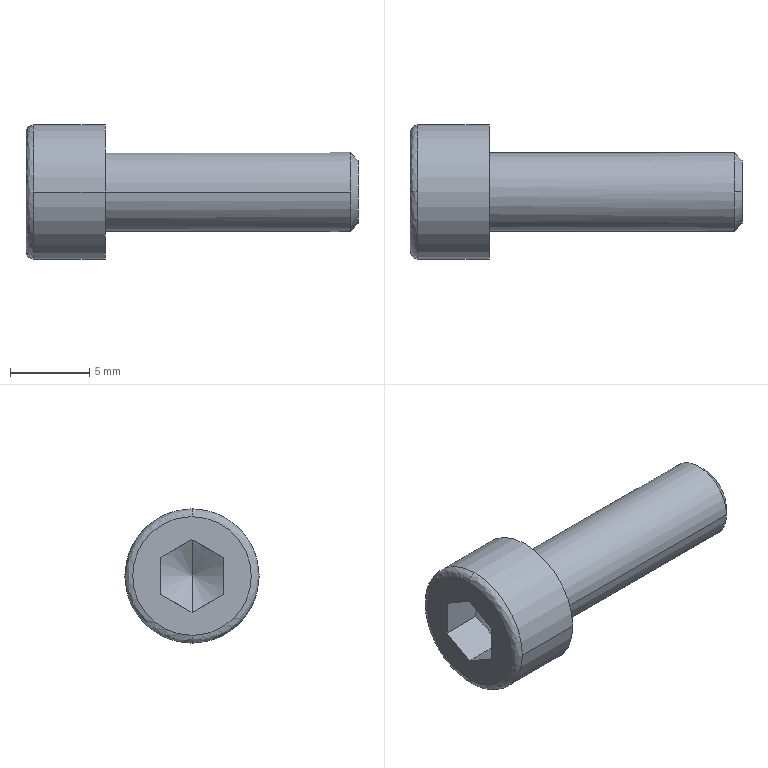Part | SolidWorks | features BaseBody 1 | 1 solid | 19 faces | box 21 x 8.5 x 8.5 mm | volume 552.853 mm3 | plane 9 | cylinder 4 | cone 4 | spline 2 | commonest cylinder face diameters 5 x2 8.5 x2
STEP:
#1=CARTESIAN_POINT('',(-4.5,0.,4.25));
#2=VERTEX_POINT('',#1);
#3=CARTESIAN_POINT('',(-4.5,-4.25,0.));
#4=VERTEX_POINT('',#3);
#5=CARTESIAN_POINT('',(-4.5,0.,0.));
#6=DIRECTION('',(1.,0.,0.));
#7=DIRECTION('',(0.,1.,0.));
#8=AXIS2_PLACEMENT_3D('',#5,#6,#7);
#9=CIRCLE('',#8,4.25);
#10=EDGE_CURVE('',#2,#4,#9,.T.);
#11=ORIENTED_EDGE('',*,*,#10,.F.);
#12=CARTESIAN_POINT('',(-5.,0.,3.75));
#13=VERTEX_POINT('',#12);
#14=CARTESIAN_POINT('',(-4.5,0.,3.75));
#15=DIRECTION('',(0.,-1.,0.));
#16=DIRECTION('',(0.,0.,1.));
#17=AXIS2_PLACEMENT_3D('',#14,#15,#16);
#18=CIRCLE('',#17,0.5);
#19=EDGE_CURVE('',#2,#13,#18,.T.);
#20=ORIENTED_EDGE('',*,*,#19,.T.);
#21=CARTESIAN_POINT('',(-5.,0.,-3.75));
#22=VERTEX_POINT('',#21);
#23=CARTESIAN_POINT('',(-5.,0.,3.75));
#24=CARTESIAN_POINT('',(-5.,-7.5,3.75));
#25=CARTESIAN_POINT('',(-5.,-7.5,-3.75));
#26=CARTESIAN_POINT('',(-5.,0.,-3.75));
#27=(BOUNDED_CURVE()B_SPLINE_CURVE(3,(#23,#24,#25,#26),.UNSPECIFIED.,.F.,.T.)B_SPLINE_CURVE_WITH_KNOTS((4,4),(0.25,0.75),.UNSPECIFIED.)CURVE()GEOMETRIC_REPRESENTATION_ITEM()RATIONAL_B_SPLINE_CURVE((1.,0.3333,0.3333,1.))REPRESENTATION_ITEM(''));
#28=EDGE_CURVE('',#13,#22,#27,.T.);
#29=ORIENTED_EDGE('',*,*,#28,.T.);
#30=CARTESIAN_POINT('',(-4.5,0.,-4.25));
#31=VERTEX_POINT('',#30);
#32=CARTESIAN_POINT('',(-4.5,0.,-3.75));
#33=DIRECTION('',(0.,1.,0.));
#34=DIRECTION('',(0.,0.,-1.));
#35=AXIS2_PLACEMENT_3D('',#32,#33,#34);
#36=CIRCLE('',#35,0.5);
#37=EDGE_CURVE('',#31,#22,#36,.T.);
#38=ORIENTED_EDGE('',*,*,#37,.F.);
#39=CARTESIAN_POINT('',(-4.5,0.,0.));
#40=DIRECTION('',(1.,0.,0.));
#41=DIRECTION('',(0.,1.,0.));
#42=AXIS2_PLACEMENT_3D('',#39,#40,#41);
#43=CIRCLE('',#42,4.25);
#44=EDGE_CURVE('',#4,#31,#43,.T.);
#45=ORIENTED_EDGE('',*,*,#44,.F.);
#46=EDGE_LOOP('',(#11,#20,#29,#38,#45));
#47=FACE_OUTER_BOUND('',#46,.T.);
#48=CARTESIAN_POINT('',(-4.5,0.,4.25));
#49=CARTESIAN_POINT('',(-4.5,-8.5,4.25));
#50=CARTESIAN_POINT('',(-4.5,-8.5,-4.25));
#51=CARTESIAN_POINT('',(-4.5,0.,-4.25));
#52=CARTESIAN_POINT('',(-4.793,0.,4.25));
#53=CARTESIAN_POINT('',(-4.793,-8.5,4.25));
#54=CARTESIAN_POINT('',(-4.793,-8.5,-4.25));
#55=CARTESIAN_POINT('',(-4.793,0.,-4.25));
#56=CARTESIAN_POINT('',(-5.,0.,4.043));
#57=CARTESIAN_POINT('',(-5.,-8.086,4.043));
#58=CARTESIAN_POINT('',(-5.,-8.086,-4.043));
#59=CARTESIAN_POINT('',(-5.,0.,-4.043));
#60=CARTESIAN_POINT('',(-5.,0.,3.75));
#61=CARTESIAN_POINT('',(-5.,-7.5,3.75));
#62=CARTESIAN_POINT('',(-5.,-7.5,-3.75));
#63=CARTESIAN_POINT('',(-5.,0.,-3.75));
#64=(BOUNDED_SURFACE()B_SPLINE_SURFACE(3,3,((#48,#49,#50,#51),(#52,#53,#54,#55),(#56,#57,#58,#59),(#60,#61,#62,#63)),.UNSPECIFIED.,.F.,.F.,.F.)B_SPLINE_SURFACE_WITH_KNOTS((4,4),(4,4),(0.,1.),(0.,1.),.UNSPECIFIED.)GEOMETRIC_REPRESENTATION_ITEM()RATIONAL_B_SPLINE_SURFACE(((1.,0.3333,0.3333,1.),(0.8047,0.2682,0.2682,0.8047),(0.8047,0.2682,0.2682,0.8047),(1.,0.3333,0.3333,1.)))REPRESENTATION_ITEM('')SURFACE());
#65=ADVANCED_FACE('',(#47),#64,.T.);
#66=CARTESIAN_POINT('',(0.,2.5,0.));
#67=VERTEX_POINT('',#66);
#68=CARTESIAN_POINT('',(0.,-2.5,0.));
#69=VERTEX_POINT('',#68);
#70=CARTESIAN_POINT('',(0.,0.,0.));
#71=DIRECTION('',(1.,0.,0.));
#72=DIRECTION('',(0.,1.,0.));
#73=AXIS2_PLACEMENT_3D('',#70,#71,#72);
#74=CIRCLE('',#73,2.5);
#75=EDGE_CURVE('',#67,#69,#74,.T.);
#76=ORIENTED_EDGE('',*,*,#75,.T.);
#77=CARTESIAN_POINT('',(15.509,-2.5,0.));
#78=VERTEX_POINT('',#77);
#79=CARTESIAN_POINT('',(9.,-2.5,0.));
#80=DIRECTION('',(1.,0.,0.));
#81=VECTOR('',#80,1000.);
#82=LINE('',#79,#81);
#83=EDGE_CURVE('',#69,#78,#82,.T.);
#84=ORIENTED_EDGE('',*,*,#83,.T.);
#85=CARTESIAN_POINT('',(15.509,0.,2.5));
#86=VERTEX_POINT('',#85);
#87=CARTESIAN_POINT('',(15.509,0.,0.));
#88=DIRECTION('',(-1.,0.,0.));
#89=DIRECTION('',(0.,1.,0.));
#90=AXIS2_PLACEMENT_3D('',#87,#88,#89);
#91=CIRCLE('',#90,2.5);
#92=EDGE_CURVE('',#78,#86,#91,.T.);
#93=ORIENTED_EDGE('',*,*,#92,.T.);
#94=CARTESIAN_POINT('',(15.509,2.5,0.));
#95=VERTEX_POINT('',#94);
#96=CARTESIAN_POINT('',(15.509,0.,0.));
#97=DIRECTION('',(-1.,0.,0.));
#98=DIRECTION('',(0.,1.,0.));
#99=AXIS2_PLACEMENT_3D('',#96,#97,#98);
#100=CIRCLE('',#99,2.5);
#101=EDGE_CURVE('',#86,#95,#100,.T.);
#102=ORIENTED_EDGE('',*,*,#101,.T.);
#103=CARTESIAN_POINT('',(9.,2.5,0.));
#104=DIRECTION('',(1.,0.,0.));
#105=VECTOR('',#104,1000.);
#106=LINE('',#103,#105);
#107=EDGE_CURVE('',#67,#95,#106,.T.);
#108=ORIENTED_EDGE('',*,*,#107,.F.);
#109=EDGE_LOOP('',(#76,#84,#93,#102,#108));
#110=FACE_OUTER_BOUND('',#109,.T.);
#111=CARTESIAN_POINT('',(9.,0.,0.));
#112=DIRECTION('',(1.,0.,0.));
#113=DIRECTION('',(0.,1.,0.));
#114=AXIS2_PLACEMENT_3D('',#111,#112,#113);
#115=CYLINDRICAL_SURFACE('',#114,2.5);
#116=ADVANCED_FACE('',(#110),#115,.T.);
#117=CARTESIAN_POINT('',(16.,0.,2.009));
#118=VERTEX_POINT('',#117);
#119=CARTESIAN_POINT('',(16.,0.,-2.009));
#120=VERTEX_POINT('',#119);
#121=CARTESIAN_POINT('',(16.,0.,0.));
#122=DIRECTION('',(-1.,0.,0.));
#123=DIRECTION('',(0.,0.,1.));
#124=AXIS2_PLACEMENT_3D('',#121,#122,#123);
#125=CIRCLE('',#124,2.009);
#126=EDGE_CURVE('',#118,#120,#125,.T.);
#127=ORIENTED_EDGE('',*,*,#126,.T.);
#128=CARTESIAN_POINT('',(15.509,0.,-2.5));
#129=VERTEX_POINT('',#128);
#130=CARTESIAN_POINT('',(15.509,0.,-2.5));
#131=DIRECTION('',(-0.7071,0.,-0.7071));
#132=VECTOR('',#131,1000.);
#133=LINE('',#130,#132);
#134=EDGE_CURVE('',#120,#129,#133,.T.);
#135=ORIENTED_EDGE('',*,*,#134,.T.);
#136=CARTESIAN_POINT('',(15.509,0.,0.));
#137=DIRECTION('',(-1.,0.,0.));
#138=DIRECTION('',(0.,1.,0.));
#139=AXIS2_PLACEMENT_3D('',#136,#137,#138);
#140=CIRCLE('',#139,2.5);
#141=EDGE_CURVE('',#95,#129,#140,.T.);
#142=ORIENTED_EDGE('',*,*,#141,.F.);
#143=ORIENTED_EDGE('',*,*,#101,.F.);
#144=CARTESIAN_POINT('',(15.509,0.,2.5));
#145=DIRECTION('',(-0.7071,0.,0.7071));
#146=VECTOR('',#145,1000.);
#147=LINE('',#144,#146);
#148=EDGE_CURVE('',#118,#86,#147,.T.);
#149=ORIENTED_EDGE('',*,*,#148,.F.);
#150=EDGE_LOOP('',(#127,#135,#142,#143,#149));
#151=FACE_OUTER_BOUND('',#150,.T.);
#152=CARTESIAN_POINT('',(15.509,0.,0.));
#153=DIRECTION('',(-1.,0.,0.));
#154=DIRECTION('',(0.,0.,1.));
#155=AXIS2_PLACEMENT_3D('',#152,#153,#154);
#156=CONICAL_SURFACE('',#155,2.5,0.7854);
#157=ADVANCED_FACE('',(#151),#156,.T.);
#158=CARTESIAN_POINT('',(-4.5,4.25,0.));
#159=VERTEX_POINT('',#158);
#160=CARTESIAN_POINT('',(-4.5,0.,0.));
#161=DIRECTION('',(1.,0.,0.));
#162=DIRECTION('',(0.,1.,0.));
#163=AXIS2_PLACEMENT_3D('',#160,#161,#162);
#164=CIRCLE('',#163,4.25);
#165=EDGE_CURVE('',#159,#2,#164,.T.);
#166=ORIENTED_EDGE('',*,*,#165,.T.);
#167=ORIENTED_EDGE('',*,*,#10,.T.);
#168=CARTESIAN_POINT('',(0.,-4.25,0.));
#169=VERTEX_POINT('',#168);
#170=CARTESIAN_POINT('',(-2.5,-4.25,0.));
#171=DIRECTION('',(1.,0.,0.));
#172=VECTOR('',#171,1000.);
#173=LINE('',#170,#172);
#174=EDGE_CURVE('',#4,#169,#173,.T.);
#175=ORIENTED_EDGE('',*,*,#174,.T.);
#176=CARTESIAN_POINT('',(0.,4.25,0.));
#177=VERTEX_POINT('',#176);
#178=CARTESIAN_POINT('',(0.,0.,0.));
#179=DIRECTION('',(1.,0.,0.));
#180=DIRECTION('',(0.,1.,0.));
#181=AXIS2_PLACEMENT_3D('',#178,#179,#180);
#182=CIRCLE('',#181,4.25);
#183=EDGE_CURVE('',#177,#169,#182,.T.);
#184=ORIENTED_EDGE('',*,*,#183,.F.);
#185=CARTESIAN_POINT('',(-2.5,4.25,0.));
#186=DIRECTION('',(1.,0.,0.));
#187=VECTOR('',#186,1000.);
#188=LINE('',#185,#187);
#189=EDGE_CURVE('',#159,#177,#188,.T.);
#190=ORIENTED_EDGE('',*,*,#189,.F.);
#191=EDGE_LOOP('',(#166,#167,#175,#184,#190));
#192=FACE_OUTER_BOUND('',#191,.T.);
#193=CARTESIAN_POINT('',(-2.5,0.,0.));
#194=DIRECTION('',(1.,0.,0.));
#195=DIRECTION('',(0.,1.,0.));
#196=AXIS2_PLACEMENT_3D('',#193,#194,#195);
#197=CYLINDRICAL_SURFACE('',#196,4.25);
#198=ADVANCED_FACE('',(#192),#197,.T.);
#199=CARTESIAN_POINT('',(-1.167,0.,0.));
#200=VERTEX_POINT('',#199);
#201=CARTESIAN_POINT('',(-2.5,0.,2.309));
#202=VERTEX_POINT('',#201);
#203=CARTESIAN_POINT('',(-2.508,0.,2.323));
#204=DIRECTION('',(-0.5,0.,0.866));
#205=VECTOR('',#204,1000.);
#206=LINE('',#203,#205);
#207=EDGE_CURVE('',#200,#202,#206,.T.);
#208=ORIENTED_EDGE('',*,*,#207,.F.);
#209=CARTESIAN_POINT('',(-2.5,0.,-2.309));
#210=VERTEX_POINT('',#209);
#211=CARTESIAN_POINT('',(-2.508,0.,-2.323));
#212=DIRECTION('',(-0.5,0.,-0.866));
#213=VECTOR('',#212,1000.);
#214=LINE('',#211,#213);
#215=EDGE_CURVE('',#200,#210,#214,.T.);
#216=ORIENTED_EDGE('',*,*,#215,.T.);
#217=CARTESIAN_POINT('',(-2.5,-2.,-1.155));
#218=VERTEX_POINT('',#217);
#219=CARTESIAN_POINT('',(-2.5,0.,-2.309));
#220=CARTESIAN_POINT('',(-2.391,-0.3266,-2.121));
#221=CARTESIAN_POINT('',(-2.322,-0.658,-1.929));
#222=CARTESIAN_POINT('',(-2.321,-1.168,-1.635));
#223=CARTESIAN_POINT('',(-2.338,-1.338,-1.537));
#224=CARTESIAN_POINT('',(-2.401,-1.672,-1.344));
#225=CARTESIAN_POINT('',(-2.446,-1.837,-1.249));
#226=CARTESIAN_POINT('',(-2.5,-2.,-1.155));
#227=B_SPLINE_CURVE_WITH_KNOTS('',3,(#219,#220,#221,#222,#223,#224,#225,#226),.UNSPECIFIED.,.F.,.F.,(4,2,2,4),(0.,0.001166,0.001749,0.002332),.UNSPECIFIED.);
#228=EDGE_CURVE('',#210,#218,#227,.T.);
#229=ORIENTED_EDGE('',*,*,#228,.T.);
#230=CARTESIAN_POINT('',(-2.5,-2.,1.155));
#231=VERTEX_POINT('',#230);
#232=CARTESIAN_POINT('',(-2.5,-2.,-1.155));
#233=CARTESIAN_POINT('',(-2.391,-2.,-0.7776));
#234=CARTESIAN_POINT('',(-2.322,-2.,-0.3949));
#235=CARTESIAN_POINT('',(-2.321,-2.,0.1941));
#236=CARTESIAN_POINT('',(-2.338,-2.,0.3903));
#237=CARTESIAN_POINT('',(-2.401,-2.,0.7756));
#238=CARTESIAN_POINT('',(-2.446,-2.,0.9659));
#239=CARTESIAN_POINT('',(-2.5,-2.,1.155));
#240=B_SPLINE_CURVE_WITH_KNOTS('',3,(#232,#233,#234,#235,#236,#237,#238,#239),.UNSPECIFIED.,.F.,.F.,(4,2,2,4),(0.,0.001166,0.001749,0.002332),.UNSPECIFIED.);
#241=EDGE_CURVE('',#218,#231,#240,.T.);
#242=ORIENTED_EDGE('',*,*,#241,.T.);
#243=CARTESIAN_POINT('',(-2.5,-2.,1.155));
#244=CARTESIAN_POINT('',(-2.391,-1.673,1.343));
#245=CARTESIAN_POINT('',(-2.322,-1.342,1.535));
#246=CARTESIAN_POINT('',(-2.321,-0.8319,1.829));
#247=CARTESIAN_POINT('',(-2.338,-0.662,1.927));
#248=CARTESIAN_POINT('',(-2.401,-0.3283,2.12));
#249=CARTESIAN_POINT('',(-2.446,-0.1635,2.215));
#250=CARTESIAN_POINT('',(-2.5,0.,2.309));
#251=B_SPLINE_CURVE_WITH_KNOTS('',3,(#243,#244,#245,#246,#247,#248,#249,#250),.UNSPECIFIED.,.F.,.F.,(4,2,2,4),(0.,0.001166,0.001749,0.002332),.UNSPECIFIED.);
#252=EDGE_CURVE('',#231,#202,#251,.T.);
#253=ORIENTED_EDGE('',*,*,#252,.T.);
#254=EDGE_LOOP('',(#208,#216,#229,#242,#253));
#255=FACE_OUTER_BOUND('',#254,.T.);
#256=CARTESIAN_POINT('',(-2.508,0.,0.));
#257=DIRECTION('',(-1.,0.,0.));
#258=DIRECTION('',(0.,0.,1.));
#259=AXIS2_PLACEMENT_3D('',#256,#257,#258);
#260=CONICAL_SURFACE('',#259,2.323,1.047);
#261=ADVANCED_FACE('',(#255),#260,.F.);
#262=ORIENTED_EDGE('',*,*,#83,.F.);
#263=CARTESIAN_POINT('',(0.,0.,0.));
#264=DIRECTION('',(1.,0.,0.));
#265=DIRECTION('',(0.,1.,0.));
#266=AXIS2_PLACEMENT_3D('',#263,#264,#265);
#267=CIRCLE('',#266,2.5);
#268=EDGE_CURVE('',#69,#67,#267,.T.);
#269=ORIENTED_EDGE('',*,*,#268,.T.);
#270=ORIENTED_EDGE('',*,*,#107,.T.);
#271=ORIENTED_EDGE('',*,*,#141,.T.);
#272=CARTESIAN_POINT('',(15.509,0.,0.));
#273=DIRECTION('',(-1.,0.,0.));
#274=DIRECTION('',(0.,1.,0.));
#275=AXIS2_PLACEMENT_3D('',#272,#273,#274);
#276=CIRCLE('',#275,2.5);
#277=EDGE_CURVE('',#129,#78,#276,.T.);
#278=ORIENTED_EDGE('',*,*,#277,.T.);
#279=EDGE_LOOP('',(#262,#269,#270,#271,#278));
#280=FACE_OUTER_BOUND('',#279,.T.);
#281=CARTESIAN_POINT('',(9.,0.,0.));
#282=DIRECTION('',(1.,0.,0.));
#283=DIRECTION('',(0.,1.,0.));
#284=AXIS2_PLACEMENT_3D('',#281,#282,#283);
#285=CYLINDRICAL_SURFACE('',#284,2.5);
#286=ADVANCED_FACE('',(#280),#285,.T.);
#287=ORIENTED_EDGE('',*,*,#134,.F.);
#288=CARTESIAN_POINT('',(16.,0.,0.));
#289=DIRECTION('',(-1.,0.,0.));
#290=DIRECTION('',(0.,0.,1.));
#291=AXIS2_PLACEMENT_3D('',#288,#289,#290);
#292=CIRCLE('',#291,2.009);
#293=EDGE_CURVE('',#120,#118,#292,.T.);
#294=ORIENTED_EDGE('',*,*,#293,.T.);
#295=ORIENTED_EDGE('',*,*,#148,.T.);
#296=ORIENTED_EDGE('',*,*,#92,.F.);
#297=ORIENTED_EDGE('',*,*,#277,.F.);
#298=EDGE_LOOP('',(#287,#294,#295,#296,#297));
#299=FACE_OUTER_BOUND('',#298,.T.);
#300=CARTESIAN_POINT('',(15.509,0.,0.));
#301=DIRECTION('',(-1.,0.,0.));
#302=DIRECTION('',(0.,0.,1.));
#303=AXIS2_PLACEMENT_3D('',#300,#301,#302);
#304=CONICAL_SURFACE('',#303,2.5,0.7854);
#305=ADVANCED_FACE('',(#299),#304,.T.);
#306=ORIENTED_EDGE('',*,*,#75,.F.);
#307=ORIENTED_EDGE('',*,*,#268,.F.);
#308=EDGE_LOOP('',(#306,#307));
#309=FACE_BOUND('',#308,.T.);
#310=ORIENTED_EDGE('',*,*,#183,.T.);
#311=CARTESIAN_POINT('',(0.,0.,0.));
#312=DIRECTION('',(1.,0.,0.));
#313=DIRECTION('',(0.,1.,0.));
#314=AXIS2_PLACEMENT_3D('',#311,#312,#313);
#315=CIRCLE('',#314,4.25);
#316=EDGE_CURVE('',#169,#177,#315,.T.);
#317=ORIENTED_EDGE('',*,*,#316,.T.);
#318=EDGE_LOOP('',(#310,#317));
#319=FACE_OUTER_BOUND('',#318,.T.);
#320=CARTESIAN_POINT('',(0.,3.375,0.));
#321=DIRECTION('',(1.,0.,0.));
#322=DIRECTION('',(0.,0.,-1.));
#323=AXIS2_PLACEMENT_3D('',#320,#321,#322);
#324=PLANE('',#323);
#325=ADVANCED_FACE('',(#309,#319),#324,.T.);
#326=ORIENTED_EDGE('',*,*,#126,.F.);
#327=ORIENTED_EDGE('',*,*,#293,.F.);
#328=EDGE_LOOP('',(#326,#327));
#329=FACE_OUTER_BOUND('',#328,.T.);
#330=CARTESIAN_POINT('',(16.,1.25,0.));
#331=DIRECTION('',(1.,0.,0.));
#332=DIRECTION('',(0.,0.,-1.));
#333=AXIS2_PLACEMENT_3D('',#330,#331,#332);
#334=PLANE('',#333);
#335=ADVANCED_FACE('',(#329),#334,.T.);
#336=ORIENTED_EDGE('',*,*,#174,.F.);
#337=ORIENTED_EDGE('',*,*,#44,.T.);
#338=CARTESIAN_POINT('',(-4.5,0.,0.));
#339=DIRECTION('',(1.,0.,0.));
#340=DIRECTION('',(0.,1.,0.));
#341=AXIS2_PLACEMENT_3D('',#338,#339,#340);
#342=CIRCLE('',#341,4.25);
#343=EDGE_CURVE('',#31,#159,#342,.T.);
#344=ORIENTED_EDGE('',*,*,#343,.T.);
#345=ORIENTED_EDGE('',*,*,#189,.T.);
#346=ORIENTED_EDGE('',*,*,#316,.F.);
#347=EDGE_LOOP('',(#336,#337,#344,#345,#346));
#348=FACE_OUTER_BOUND('',#347,.T.);
#349=CARTESIAN_POINT('',(-2.5,0.,0.));
#350=DIRECTION('',(1.,0.,0.));
#351=DIRECTION('',(0.,1.,0.));
#352=AXIS2_PLACEMENT_3D('',#349,#350,#351);
#353=CYLINDRICAL_SURFACE('',#352,4.25);
#354=ADVANCED_FACE('',(#348),#353,.T.);
#355=ORIENTED_EDGE('',*,*,#19,.F.);
#356=ORIENTED_EDGE('',*,*,#165,.F.);
#357=ORIENTED_EDGE('',*,*,#343,.F.);
#358=ORIENTED_EDGE('',*,*,#37,.T.);
#359=CARTESIAN_POINT('',(-5.,0.,-3.75));
#360=CARTESIAN_POINT('',(-5.,7.5,-3.75));
#361=CARTESIAN_POINT('',(-5.,7.5,3.75));
#362=CARTESIAN_POINT('',(-5.,0.,3.75));
#363=(BOUNDED_CURVE()B_SPLINE_CURVE(3,(#359,#360,#361,#362),.UNSPECIFIED.,.F.,.T.)B_SPLINE_CURVE_WITH_KNOTS((4,4),(0.75,1.25),.UNSPECIFIED.)CURVE()GEOMETRIC_REPRESENTATION_ITEM()RATIONAL_B_SPLINE_CURVE((1.,0.3333,0.3333,1.))REPRESENTATION_ITEM(''));
#364=EDGE_CURVE('',#22,#13,#363,.T.);
#365=ORIENTED_EDGE('',*,*,#364,.T.);
#366=EDGE_LOOP('',(#355,#356,#357,#358,#365));
#367=FACE_OUTER_BOUND('',#366,.T.);
#368=CARTESIAN_POINT('',(-4.5,0.,-4.25));
#369=CARTESIAN_POINT('',(-4.5,8.5,-4.25));
#370=CARTESIAN_POINT('',(-4.5,8.5,4.25));
#371=CARTESIAN_POINT('',(-4.5,0.,4.25));
#372=CARTESIAN_POINT('',(-4.793,0.,-4.25));
#373=CARTESIAN_POINT('',(-4.793,8.5,-4.25));
#374=CARTESIAN_POINT('',(-4.793,8.5,4.25));
#375=CARTESIAN_POINT('',(-4.793,0.,4.25));
#376=CARTESIAN_POINT('',(-5.,0.,-4.043));
#377=CARTESIAN_POINT('',(-5.,8.086,-4.043));
#378=CARTESIAN_POINT('',(-5.,8.086,4.043));
#379=CARTESIAN_POINT('',(-5.,0.,4.043));
#380=CARTESIAN_POINT('',(-5.,0.,-3.75));
#381=CARTESIAN_POINT('',(-5.,7.5,-3.75));
#382=CARTESIAN_POINT('',(-5.,7.5,3.75));
#383=CARTESIAN_POINT('',(-5.,0.,3.75));
#384=(BOUNDED_SURFACE()B_SPLINE_SURFACE(3,3,((#368,#369,#370,#371),(#372,#373,#374,#375),(#376,#377,#378,#379),(#380,#381,#382,#383)),.UNSPECIFIED.,.F.,.F.,.F.)B_SPLINE_SURFACE_WITH_KNOTS((4,4),(4,4),(0.,1.),(0.,1.),.UNSPECIFIED.)GEOMETRIC_REPRESENTATION_ITEM()RATIONAL_B_SPLINE_SURFACE(((1.,0.3333,0.3333,1.),(0.8047,0.2682,0.2682,0.8047),(0.8047,0.2682,0.2682,0.8047),(1.,0.3333,0.3333,1.)))REPRESENTATION_ITEM('')SURFACE());
#385=ADVANCED_FACE('',(#367),#384,.T.);
#386=CARTESIAN_POINT('',(-5.,-2.,-1.155));
#387=VERTEX_POINT('',#386);
#388=CARTESIAN_POINT('',(-5.,0.,-2.309));
#389=VERTEX_POINT('',#388);
#390=CARTESIAN_POINT('',(-5.,-2.,-1.155));
#391=DIRECTION('',(0.,0.866,-0.5));
#392=VECTOR('',#391,1000.);
#393=LINE('',#390,#392);
#394=EDGE_CURVE('',#387,#389,#393,.T.);
#395=ORIENTED_EDGE('',*,*,#394,.T.);
#396=CARTESIAN_POINT('',(-5.,2.,-1.155));
#397=VERTEX_POINT('',#396);
#398=CARTESIAN_POINT('',(-5.,0.,-2.309));
#399=DIRECTION('',(0.,0.866,0.5));
#400=VECTOR('',#399,1000.);
#401=LINE('',#398,#400);
#402=EDGE_CURVE('',#389,#397,#401,.T.);
#403=ORIENTED_EDGE('',*,*,#402,.T.);
#404=CARTESIAN_POINT('',(-5.,2.,1.155));
#405=VERTEX_POINT('',#404);
#406=CARTESIAN_POINT('',(-5.,2.,0.));
#407=DIRECTION('',(0.,0.,1.));
#408=VECTOR('',#407,1000.);
#409=LINE('',#406,#408);
#410=EDGE_CURVE('',#397,#405,#409,.T.);
#411=ORIENTED_EDGE('',*,*,#410,.T.);
#412=CARTESIAN_POINT('',(-5.,0.,2.309));
#413=VERTEX_POINT('',#412);
#414=CARTESIAN_POINT('',(-5.,2.,1.155));
#415=DIRECTION('',(0.,-0.866,0.5));
#416=VECTOR('',#415,1000.);
#417=LINE('',#414,#416);
#418=EDGE_CURVE('',#405,#413,#417,.T.);
#419=ORIENTED_EDGE('',*,*,#418,.T.);
#420=CARTESIAN_POINT('',(-5.,-2.,1.155));
#421=VERTEX_POINT('',#420);
#422=CARTESIAN_POINT('',(-5.,0.,2.309));
#423=DIRECTION('',(0.,-0.866,-0.5));
#424=VECTOR('',#423,1000.);
#425=LINE('',#422,#424);
#426=EDGE_CURVE('',#413,#421,#425,.T.);
#427=ORIENTED_EDGE('',*,*,#426,.T.);
#428=CARTESIAN_POINT('',(-5.,-2.,0.));
#429=DIRECTION('',(0.,0.,-1.));
#430=VECTOR('',#429,1000.);
#431=LINE('',#428,#430);
#432=EDGE_CURVE('',#421,#387,#431,.T.);
#433=ORIENTED_EDGE('',*,*,#432,.T.);
#434=EDGE_LOOP('',(#395,#403,#411,#419,#427,#433));
#435=FACE_BOUND('',#434,.T.);
#436=ORIENTED_EDGE('',*,*,#364,.F.);
#437=ORIENTED_EDGE('',*,*,#28,.F.);
#438=EDGE_LOOP('',(#436,#437));
#439=FACE_OUTER_BOUND('',#438,.T.);
#440=CARTESIAN_POINT('',(-5.,3.28,0.));
#441=DIRECTION('',(-1.,0.,0.));
#442=DIRECTION('',(0.,0.,1.));
#443=AXIS2_PLACEMENT_3D('',#440,#441,#442);
#444=PLANE('',#443);
#445=ADVANCED_FACE('',(#435,#439),#444,.T.);
#446=CARTESIAN_POINT('',(-2.5,2.,-1.155));
#447=VERTEX_POINT('',#446);
#448=CARTESIAN_POINT('',(-5.,2.,-1.155));
#449=DIRECTION('',(1.,0.,0.));
#450=VECTOR('',#449,1000.);
#451=LINE('',#448,#450);
#452=EDGE_CURVE('',#397,#447,#451,.T.);
#453=ORIENTED_EDGE('',*,*,#452,.F.);
#454=ORIENTED_EDGE('',*,*,#402,.F.);
#455=CARTESIAN_POINT('',(-5.,0.,-2.309));
#456=DIRECTION('',(-1.,0.,0.));
#457=VECTOR('',#456,1000.);
#458=LINE('',#455,#457);
#459=EDGE_CURVE('',#210,#389,#458,.T.);
#460=ORIENTED_EDGE('',*,*,#459,.F.);
#461=CARTESIAN_POINT('',(-2.5,2.,-1.155));
#462=CARTESIAN_POINT('',(-2.391,1.673,-1.343));
#463=CARTESIAN_POINT('',(-2.322,1.342,-1.535));
#464=CARTESIAN_POINT('',(-2.321,0.8319,-1.829));
#465=CARTESIAN_POINT('',(-2.338,0.662,-1.927));
#466=CARTESIAN_POINT('',(-2.401,0.3283,-2.12));
#467=CARTESIAN_POINT('',(-2.446,0.1635,-2.215));
#468=CARTESIAN_POINT('',(-2.5,0.,-2.309));
#469=B_SPLINE_CURVE_WITH_KNOTS('',3,(#461,#462,#463,#464,#465,#466,#467,#468),.UNSPECIFIED.,.F.,.F.,(4,2,2,4),(0.,0.001166,0.001749,0.002332),.UNSPECIFIED.);
#470=EDGE_CURVE('',#447,#210,#469,.T.);
#471=ORIENTED_EDGE('',*,*,#470,.F.);
#472=EDGE_LOOP('',(#453,#454,#460,#471));
#473=FACE_OUTER_BOUND('',#472,.T.);
#474=CARTESIAN_POINT('',(-5.,2.,-1.155));
#475=DIRECTION('',(0.,0.5,-0.866));
#476=DIRECTION('',(0.,0.866,0.5));
#477=AXIS2_PLACEMENT_3D('',#474,#475,#476);
#478=PLANE('',#477);
#479=ADVANCED_FACE('',(#473),#478,.F.);
#480=ORIENTED_EDGE('',*,*,#459,.T.);
#481=ORIENTED_EDGE('',*,*,#394,.F.);
#482=CARTESIAN_POINT('',(-5.,-2.,-1.155));
#483=DIRECTION('',(-1.,0.,0.));
#484=VECTOR('',#483,1000.);
#485=LINE('',#482,#484);
#486=EDGE_CURVE('',#218,#387,#485,.T.);
#487=ORIENTED_EDGE('',*,*,#486,.F.);
#488=ORIENTED_EDGE('',*,*,#228,.F.);
#489=EDGE_LOOP('',(#480,#481,#487,#488));
#490=FACE_OUTER_BOUND('',#489,.T.);
#491=CARTESIAN_POINT('',(-5.,0.,-2.309));
#492=DIRECTION('',(0.,-0.5,-0.866));
#493=DIRECTION('',(0.,0.866,-0.5));
#494=AXIS2_PLACEMENT_3D('',#491,#492,#493);
#495=PLANE('',#494);
#496=ADVANCED_FACE('',(#490),#495,.F.);
#497=ORIENTED_EDGE('',*,*,#486,.T.);
#498=ORIENTED_EDGE('',*,*,#432,.F.);
#499=CARTESIAN_POINT('',(-5.,-2.,1.155));
#500=DIRECTION('',(-1.,0.,0.));
#501=VECTOR('',#500,1000.);
#502=LINE('',#499,#501);
#503=EDGE_CURVE('',#231,#421,#502,.T.);
#504=ORIENTED_EDGE('',*,*,#503,.F.);
#505=ORIENTED_EDGE('',*,*,#241,.F.);
#506=EDGE_LOOP('',(#497,#498,#504,#505));
#507=FACE_OUTER_BOUND('',#506,.T.);
#508=CARTESIAN_POINT('',(-5.,-2.,-1.155));
#509=DIRECTION('',(0.,-1.,0.));
#510=DIRECTION('',(0.,0.,-1.));
#511=AXIS2_PLACEMENT_3D('',#508,#509,#510);
#512=PLANE('',#511);
#513=ADVANCED_FACE('',(#507),#512,.F.);
#514=ORIENTED_EDGE('',*,*,#503,.T.);
#515=ORIENTED_EDGE('',*,*,#426,.F.);
#516=CARTESIAN_POINT('',(-5.,0.,2.309));
#517=DIRECTION('',(-1.,0.,0.));
#518=VECTOR('',#517,1000.);
#519=LINE('',#516,#518);
#520=EDGE_CURVE('',#202,#413,#519,.T.);
#521=ORIENTED_EDGE('',*,*,#520,.F.);
#522=ORIENTED_EDGE('',*,*,#252,.F.);
#523=EDGE_LOOP('',(#514,#515,#521,#522));
#524=FACE_OUTER_BOUND('',#523,.T.);
#525=CARTESIAN_POINT('',(-5.,-2.,1.155));
#526=DIRECTION('',(0.,-0.5,0.866));
#527=DIRECTION('',(0.,-0.866,-0.5));
#528=AXIS2_PLACEMENT_3D('',#525,#526,#527);
#529=PLANE('',#528);
#530=ADVANCED_FACE('',(#524),#529,.F.);
#531=ORIENTED_EDGE('',*,*,#520,.T.);
#532=ORIENTED_EDGE('',*,*,#418,.F.);
#533=CARTESIAN_POINT('',(-2.5,2.,1.155));
#534=VERTEX_POINT('',#533);
#535=CARTESIAN_POINT('',(-5.,2.,1.155));
#536=DIRECTION('',(-1.,0.,0.));
#537=VECTOR('',#536,1000.);
#538=LINE('',#535,#537);
#539=EDGE_CURVE('',#534,#405,#538,.T.);
#540=ORIENTED_EDGE('',*,*,#539,.F.);
#541=CARTESIAN_POINT('',(-2.5,0.,2.309));
#542=CARTESIAN_POINT('',(-2.391,0.3266,2.121));
#543=CARTESIAN_POINT('',(-2.322,0.658,1.929));
#544=CARTESIAN_POINT('',(-2.321,1.168,1.635));
#545=CARTESIAN_POINT('',(-2.338,1.338,1.537));
#546=CARTESIAN_POINT('',(-2.401,1.672,1.344));
#547=CARTESIAN_POINT('',(-2.446,1.837,1.249));
#548=CARTESIAN_POINT('',(-2.5,2.,1.155));
#549=B_SPLINE_CURVE_WITH_KNOTS('',3,(#541,#542,#543,#544,#545,#546,#547,#548),.UNSPECIFIED.,.F.,.F.,(4,2,2,4),(0.,0.001166,0.001749,0.002332),.UNSPECIFIED.);
#550=EDGE_CURVE('',#202,#534,#549,.T.);
#551=ORIENTED_EDGE('',*,*,#550,.F.);
#552=EDGE_LOOP('',(#531,#532,#540,#551));
#553=FACE_OUTER_BOUND('',#552,.T.);
#554=CARTESIAN_POINT('',(-5.,0.,2.309));
#555=DIRECTION('',(0.,0.5,0.866));
#556=DIRECTION('',(0.,-0.866,0.5));
#557=AXIS2_PLACEMENT_3D('',#554,#555,#556);
#558=PLANE('',#557);
#559=ADVANCED_FACE('',(#553),#558,.F.);
#560=ORIENTED_EDGE('',*,*,#539,.T.);
#561=ORIENTED_EDGE('',*,*,#410,.F.);
#562=ORIENTED_EDGE('',*,*,#452,.T.);
#563=CARTESIAN_POINT('',(-2.5,2.,1.155));
#564=CARTESIAN_POINT('',(-2.391,2.,0.7776));
#565=CARTESIAN_POINT('',(-2.322,2.,0.3949));
#566=CARTESIAN_POINT('',(-2.321,2.,-0.1941));
#567=CARTESIAN_POINT('',(-2.338,2.,-0.3903));
#568=CARTESIAN_POINT('',(-2.401,2.,-0.7756));
#569=CARTESIAN_POINT('',(-2.446,2.,-0.9659));
#570=CARTESIAN_POINT('',(-2.5,2.,-1.155));
#571=B_SPLINE_CURVE_WITH_KNOTS('',3,(#563,#564,#565,#566,#567,#568,#569,#570),.UNSPECIFIED.,.F.,.F.,(4,2,2,4),(0.,0.001166,0.001749,0.002332),.UNSPECIFIED.);
#572=EDGE_CURVE('',#534,#447,#571,.T.);
#573=ORIENTED_EDGE('',*,*,#572,.F.);
#574=EDGE_LOOP('',(#560,#561,#562,#573));
#575=FACE_OUTER_BOUND('',#574,.T.);
#576=CARTESIAN_POINT('',(-5.,2.,1.155));
#577=DIRECTION('',(0.,1.,0.));
#578=DIRECTION('',(0.,0.,1.));
#579=AXIS2_PLACEMENT_3D('',#576,#577,#578);
#580=PLANE('',#579);
#581=ADVANCED_FACE('',(#575),#580,.F.);
#582=ORIENTED_EDGE('',*,*,#215,.F.);
#583=ORIENTED_EDGE('',*,*,#207,.T.);
#584=ORIENTED_EDGE('',*,*,#550,.T.);
#585=ORIENTED_EDGE('',*,*,#572,.T.);
#586=ORIENTED_EDGE('',*,*,#470,.T.);
#587=EDGE_LOOP('',(#582,#583,#584,#585,#586));
#588=FACE_OUTER_BOUND('',#587,.T.);
#589=CARTESIAN_POINT('',(-2.508,0.,0.));
#590=DIRECTION('',(-1.,0.,0.));
#591=DIRECTION('',(0.,0.,1.));
#592=AXIS2_PLACEMENT_3D('',#589,#590,#591);
#593=CONICAL_SURFACE('',#592,2.323,1.047);
#594=ADVANCED_FACE('',(#588),#593,.F.);
#595=CLOSED_SHELL('',(#65,#116,#157,#198,#261,#286,#305,#325,#335,#354,#385,#445,#479,#496,#513,#530,#559,#581,#594));
#596=MANIFOLD_SOLID_BREP('',#595);
#597=CARTESIAN_POINT('',(0.,0.,0.));
#598=DIRECTION('',(0.,0.,1.));
#599=DIRECTION('',(1.,0.,0.));
#600=AXIS2_PLACEMENT_3D('',#597,#598,#599);
#601=(LENGTH_UNIT()NAMED_UNIT(*)SI_UNIT(.MILLI.,.METRE.));
#602=UNCERTAINTY_MEASURE_WITH_UNIT(LENGTH_MEASURE(0.00001),#601,'','');
#603=(NAMED_UNIT(*)PLANE_ANGLE_UNIT()SI_UNIT($,.RADIAN.));
#604=(NAMED_UNIT(*)SI_UNIT($,.STERADIAN.)SOLID_ANGLE_UNIT());
#605=(GEOMETRIC_REPRESENTATION_CONTEXT(3)GLOBAL_UNCERTAINTY_ASSIGNED_CONTEXT((#602))GLOBAL_UNIT_ASSIGNED_CONTEXT((#601,#603,#604))REPRESENTATION_CONTEXT('',''));
#606=ADVANCED_BREP_SHAPE_REPRESENTATION('',(#596,#600),#605);